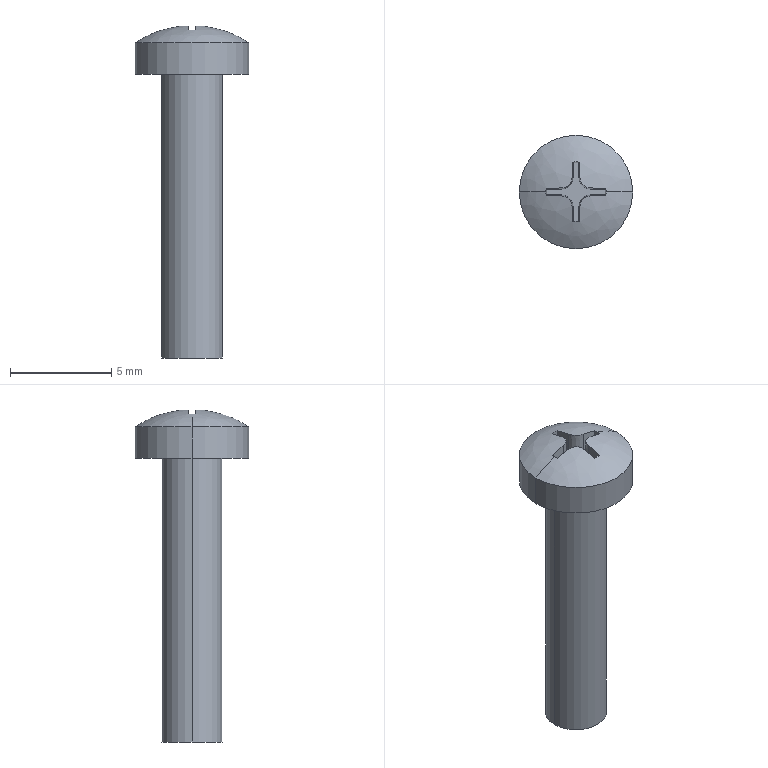Part | STEP file | GB818-M3X14-ZN-4.8_1 | 1 solid | 26 faces | box 5.6 x 5.6 x 16.376 mm | volume 144.849 mm3 | plane 11 | cone 9 | cylinder 4 | spline 2 | commonest cylinder face diameters 3 x2 5.6 x2